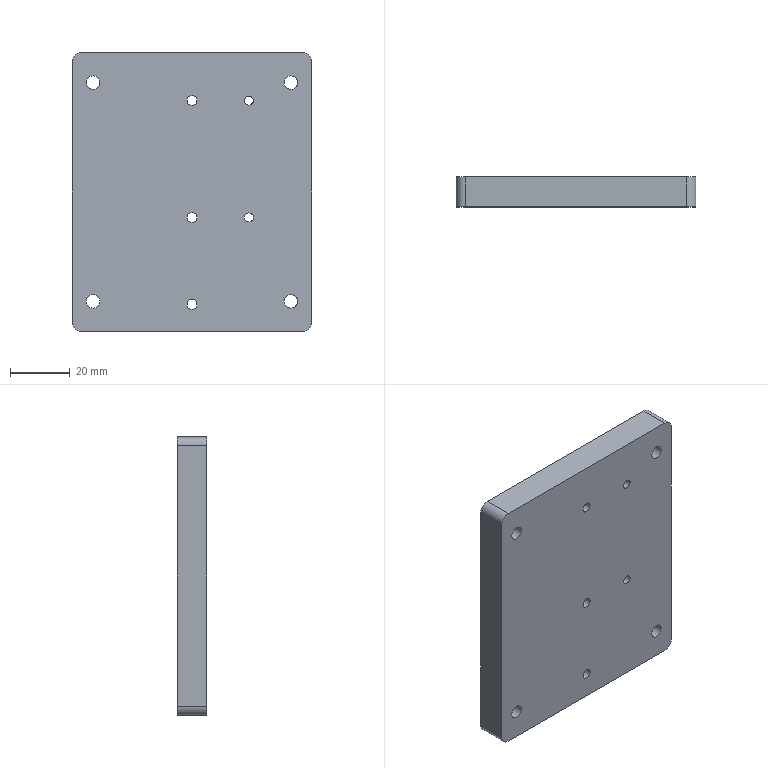CAM job | NX | 3+2 milling, drilling | part box 80 x 10 x 93 mm | stock box 85 x 12 x 98 mm
Tools:
number,name,description,diameter,corner_radius,flute_length,length,flutes
18,D2,平底铣刀-粗,2.0,0.0,50.0,75.0,2
4,D4,平底铣刀-粗,4.0,0.0,25.0,75.0,2
9,D10,平底铣刀-粗,10.0,0.0,35.0,75.0,2
19,D2-J,平底铣刀-精,2.0,0.0,50.0,75.0,2
10,D10-J,平底铣刀-精,10.0,0.0,35.0,75.0,2
1,D80R0.8_FLYCUTTER,圆鼻刀-粗,80.0,0.8,50.0,75.0,2
1,D80R0.8_FLYCUTTER-J,圆鼻刀-精,80.0,0.8,50.0,75.0,2
2,D6_CHAMFER,倒角刀,6.0,0.0,3.0,25.0,2
21,M4X0.7,丝锥,3.3,0.0,35.0,50.0,2
17,ZT3,钻头,3.0,0.0,35.0,50.0,2
11,ZT4.5,钻头,4.5,0.0,35.0,50.0,2
13,DRILL3.3,Twist Drill 3.3 mm,3.3,0.0,35.0,35.008,2
Operations:
program,operation,operation_type,tool,method,geometry_group,spindle_rpm,surface_speed,feed_per_tooth,feed_cut,feed_plunge,cut_length_mm,path_length_mm,cut_time_min,machine_time_min
B,BOTTOMWALL_FACEROUGH_COPY,VolumeBased25DMillingOperation,D80R0.8_FLYCUTTER,LAYER_ROUGH-DEPTHK-STEPG,W-B,2800.0,703.696,0.5357,3000.0,100.0,1570.79,1679.679,0.5236,0.5345
B,BOTTOMWALL_FACEFINISH_COPY,VolumeBased25DMillingOperation,D80R0.8_FLYCUTTER-J,SIDEMILL_FINISH-DEPTHK-STEPG,W-B,4000.0,1005.28,0.125,1000.0,100.0,392.11,428.11,0.3921,0.3957
B,DRILL_CHAMFER_3,Operation,D6_CHAMFER,METHOD,W-B,8000.0,150.796,0.0625,1000.0,0.0,9.6,101.315,0.0096,0.0188
B,DRILL_CHAMFER_4,Operation,D6_CHAMFER,METHOD,W-B,8000.0,150.796,0.0625,1000.0,0.0,22.2,298.598,0.0222,0.0498
B,DRILL_CHAMFER_5,Operation,D6_CHAMFER,METHOD,W-B,8000.0,150.796,0.0625,1000.0,0.0,15.6,145.47,0.0156,0.0286
B,C0.3_CLOSEDCONTOUR_CHAMFER6X45L_COPY,PlanarMilling,D6_CHAMFER,CLIMB_CHAMFER-DEPTH0-STEPG,W-B,7000.0,131.0,0.1071,1500.0,100.0,358.481,394.481,0.239,0.2426
A,TOPFACE,FaceMilling,D80R0.8_FLYCUTTER,SIDEMILL_FINISH-DEPTHK-STEPG,W-A,4000.0,1005.31,0.125,1000.0,100.0,413.333,449.333,0.4133,0.4169
A,PROFILE_ROUGH_2,VolumeBased25DMillingOperation,D10,METHOD,W-A,8000.0,251.327,0.3125,5000.0,80.0,5594.918,5643.518,1.119,1.124
A,SPOT_DEPTH0.8,Operation,D6_CHAMFER,NONE,W-A,8000.0,150.796,0.0312,500.0,90.0,16.2,320.466,0.0324,0.0628
A,THRUHOLE_M4_TAPDRILL,Operation,DRILL3.3,NONE,W-A,3000.0,31.102,0.05,300.0,90.0,50.974,211.979,0.1699,0.186
A,THRUHOLE_FINISH4.0_PREDRILL,Operation,ZT3,NONE,W-A,3000.0,36.757,0.0417,250.0,90.0,29.803,139.618,0.1192,0.1302
A,CSINK_DRILL_SEG0,Operation,ZT4.5,NONE,W-A,2800.0,39.584,0.0179,100.0,90.0,57.408,362.837,0.5741,0.6046
A,HOLEMILL_ROUGH_D4_1,CylinderMilling,D4,NONE,W-A,8000.0,100.531,0.075,1200.0,100.0,851.827,1232.427,0.7099,0.7479
A,HOLEMILL_FINISH_D4_1,CylinderMilling,D4,FINISH_STEPDEPTH_OFF,W-A,8000.0,100.531,0.0312,500.0,100.0,128.184,508.784,0.2564,0.2944
A,HOLEMILL_ROUGH_D2_1,CylinderMilling,D2,NONE,W-A,8000.0,50.266,0.0375,600.0,100.0,330.926,458.526,0.5515,0.5643
A,SELBODYONLY,SurfaceContour,D6_CHAMFER,METHOD,W-A,8000.0,150.796,0.1875,3000.0,100.0,358.163,393.964,0.1194,0.123
A,DRILL_CHAMFER_1,Operation,D6_CHAMFER,METHOD,W-A,8000.0,150.796,0.0312,500.0,0.0,15.6,145.47,0.0312,0.0442
A,DRILL_CHAMFER_2,Operation,D6_CHAMFER,METHOD,W-A,8000.0,150.796,0.0312,500.0,0.0,10.6,103.315,0.0212,0.0305
A,MILL_CHAMFER_1,PlanarMilling,D6_CHAMFER,NONE,W-A,8000.0,150.796,0.0312,500.0,100.0,135.871,479.043,0.2717,0.3061
A,HOLEMILL_FINISH_D2_1,CylinderMilling,D2-J,FINISH_STEPDEPTH_OFF,W-A,8000.0,50.266,0.0125,200.0,100.0,86.928,214.528,0.4346,0.4474
A,THRUHOLE_TAP_M4,Operation,M4X0.7,METHOD,W-A,600.0,6.22,0.0006,0.7,90.0,42.0,194.03,60.0,60.015
A,PROFILE_SEMI_2,VolumeBased25DMillingOperation,D10-J,METHOD,W-A,8000.0,251.327,0.0625,1000.0,100.0,377.252,436.452,0.3773,0.3832